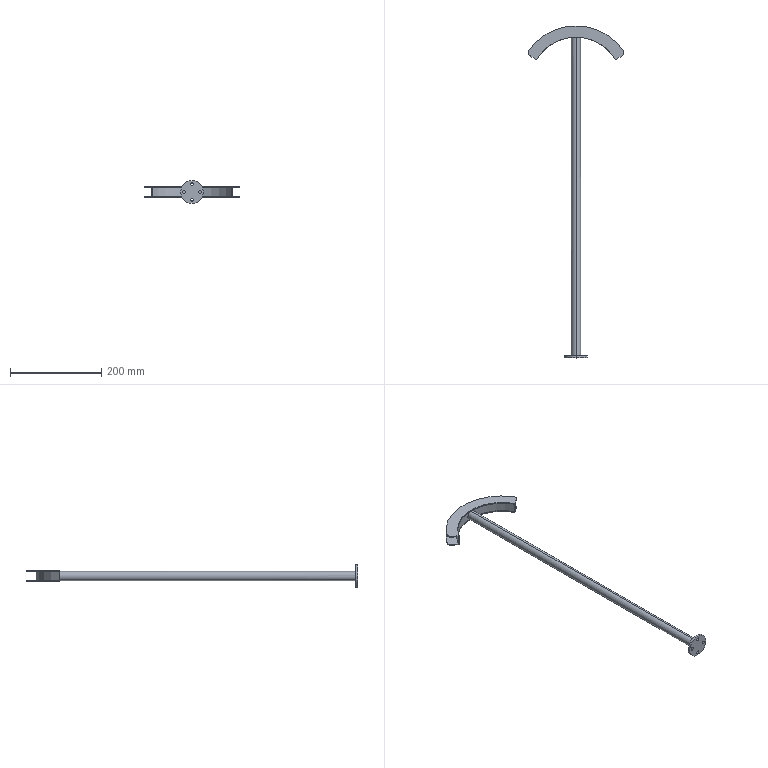Part | STEP file | TJ-DHQM-003-014 | 3 solids | 43 faces | box 208.431 x 730 x 50 mm | volume 102076 mm3 | cylinder 28 | plane 15 | commonest cylinder face diameters 6 x8 20 x8 200 x5 17 x2 50 x2 250 x2
STEP:
#1=CARTESIAN_POINT('',(104.216,65.942,-2.));
#2=VERTEX_POINT('',#1);
#3=CARTESIAN_POINT('',(99.216,57.282,-2.));
#4=VERTEX_POINT('',#3);
#5=CARTESIAN_POINT('',(94.216,65.942,-2.));
#6=DIRECTION('',(0.,0.,-1.));
#7=DIRECTION('',(-1.,0.,0.));
#8=AXIS2_PLACEMENT_3D('',#5,#6,#7);
#9=CIRCLE('',#8,10.);
#10=EDGE_CURVE('',#2,#4,#9,.T.);
#11=ORIENTED_EDGE('',*,*,#10,.F.);
#12=CARTESIAN_POINT('',(104.216,65.942,0.));
#13=VERTEX_POINT('',#12);
#14=CARTESIAN_POINT('',(104.216,65.942,-2.));
#15=DIRECTION('',(0.,0.,1.));
#16=VECTOR('',#15,1000.);
#17=LINE('',#14,#16);
#18=EDGE_CURVE('',#2,#13,#17,.T.);
#19=ORIENTED_EDGE('',*,*,#18,.T.);
#20=CARTESIAN_POINT('',(99.216,57.282,0.));
#21=VERTEX_POINT('',#20);
#22=CARTESIAN_POINT('',(94.216,65.942,0.));
#23=DIRECTION('',(0.,0.,1.));
#24=DIRECTION('',(-1.,0.,0.));
#25=AXIS2_PLACEMENT_3D('',#22,#23,#24);
#26=CIRCLE('',#25,10.);
#27=EDGE_CURVE('',#21,#13,#26,.T.);
#28=ORIENTED_EDGE('',*,*,#27,.F.);
#29=CARTESIAN_POINT('',(99.216,57.282,-2.));
#30=DIRECTION('',(0.,0.,1.));
#31=VECTOR('',#30,1000.);
#32=LINE('',#29,#31);
#33=EDGE_CURVE('',#4,#21,#32,.T.);
#34=ORIENTED_EDGE('',*,*,#33,.F.);
#35=EDGE_LOOP('',(#11,#19,#28,#34));
#36=FACE_OUTER_BOUND('',#35,.T.);
#37=CARTESIAN_POINT('',(94.216,65.942,-2.));
#38=DIRECTION('',(0.,0.,1.));
#39=DIRECTION('',(1.,0.,0.));
#40=AXIS2_PLACEMENT_3D('',#37,#38,#39);
#41=CYLINDRICAL_SURFACE('',#40,10.);
#42=ADVANCED_FACE('',(#36),#41,.T.);
#43=CARTESIAN_POINT('',(-102.408,71.677,0.));
#44=VERTEX_POINT('',#43);
#45=CARTESIAN_POINT('',(102.408,71.677,0.));
#46=VERTEX_POINT('',#45);
#47=CARTESIAN_POINT('',(0.,0.,0.));
#48=DIRECTION('',(0.,0.,-1.));
#49=DIRECTION('',(-1.,0.,0.));
#50=AXIS2_PLACEMENT_3D('',#47,#48,#49);
#51=CIRCLE('',#50,125.);
#52=EDGE_CURVE('',#44,#46,#51,.T.);
#53=ORIENTED_EDGE('',*,*,#52,.T.);
#54=CARTESIAN_POINT('',(102.408,71.677,-2.));
#55=VERTEX_POINT('',#54);
#56=CARTESIAN_POINT('',(102.408,71.677,-2.));
#57=DIRECTION('',(0.,0.,-1.));
#58=VECTOR('',#57,1000.);
#59=LINE('',#56,#58);
#60=EDGE_CURVE('',#46,#55,#59,.T.);
#61=ORIENTED_EDGE('',*,*,#60,.T.);
#62=CARTESIAN_POINT('',(-102.408,71.677,-2.));
#63=VERTEX_POINT('',#62);
#64=CARTESIAN_POINT('',(0.,0.,-2.));
#65=DIRECTION('',(0.,0.,-1.));
#66=DIRECTION('',(-1.,0.,0.));
#67=AXIS2_PLACEMENT_3D('',#64,#65,#66);
#68=CIRCLE('',#67,125.);
#69=EDGE_CURVE('',#63,#55,#68,.T.);
#70=ORIENTED_EDGE('',*,*,#69,.F.);
#71=CARTESIAN_POINT('',(-102.408,71.677,-2.));
#72=DIRECTION('',(0.,0.,1.));
#73=VECTOR('',#72,1000.);
#74=LINE('',#71,#73);
#75=EDGE_CURVE('',#63,#44,#74,.T.);
#76=ORIENTED_EDGE('',*,*,#75,.T.);
#77=EDGE_LOOP('',(#53,#61,#70,#76));
#78=FACE_OUTER_BOUND('',#77,.T.);
#79=CARTESIAN_POINT('',(0.,0.,-2.));
#80=DIRECTION('',(0.,0.,1.));
#81=DIRECTION('',(1.,0.,0.));
#82=AXIS2_PLACEMENT_3D('',#79,#80,#81);
#83=CYLINDRICAL_SURFACE('',#82,125.);
#84=ADVANCED_FACE('',(#78),#83,.T.);
#85=CARTESIAN_POINT('',(86.603,50.,-2.));
#86=VERTEX_POINT('',#85);
#87=CARTESIAN_POINT('',(108.253,62.5,-2.));
#88=DIRECTION('',(-0.866,-0.5,0.));
#89=VECTOR('',#88,1000.);
#90=LINE('',#87,#89);
#91=EDGE_CURVE('',#4,#86,#90,.T.);
#92=ORIENTED_EDGE('',*,*,#91,.F.);
#93=ORIENTED_EDGE('',*,*,#33,.T.);
#94=CARTESIAN_POINT('',(86.603,50.,0.));
#95=VERTEX_POINT('',#94);
#96=CARTESIAN_POINT('',(108.253,62.5,0.));
#97=DIRECTION('',(-0.866,-0.5,0.));
#98=VECTOR('',#97,1000.);
#99=LINE('',#96,#98);
#100=EDGE_CURVE('',#21,#95,#99,.T.);
#101=ORIENTED_EDGE('',*,*,#100,.T.);
#102=CARTESIAN_POINT('',(86.603,50.,-2.));
#103=DIRECTION('',(0.,0.,1.));
#104=VECTOR('',#103,1000.);
#105=LINE('',#102,#104);
#106=EDGE_CURVE('',#86,#95,#105,.T.);
#107=ORIENTED_EDGE('',*,*,#106,.F.);
#108=EDGE_LOOP('',(#92,#93,#101,#107));
#109=FACE_OUTER_BOUND('',#108,.T.);
#110=CARTESIAN_POINT('',(108.253,62.5,-2.));
#111=DIRECTION('',(-0.5,0.866,0.));
#112=DIRECTION('',(-0.866,-0.5,0.));
#113=AXIS2_PLACEMENT_3D('',#110,#111,#112);
#114=PLANE('',#113);
#115=ADVANCED_FACE('',(#109),#114,.F.);
#116=CARTESIAN_POINT('',(-86.603,50.,0.));
#117=VERTEX_POINT('',#116);
#118=CARTESIAN_POINT('',(0.,0.,0.));
#119=DIRECTION('',(0.,0.,1.));
#120=DIRECTION('',(-1.,0.,0.));
#121=AXIS2_PLACEMENT_3D('',#118,#119,#120);
#122=CIRCLE('',#121,100.);
#123=EDGE_CURVE('',#95,#117,#122,.T.);
#124=ORIENTED_EDGE('',*,*,#123,.T.);
#125=CARTESIAN_POINT('',(-86.603,50.,-2.));
#126=VERTEX_POINT('',#125);
#127=CARTESIAN_POINT('',(-86.603,50.,-2.));
#128=DIRECTION('',(0.,0.,1.));
#129=VECTOR('',#128,1000.);
#130=LINE('',#127,#129);
#131=EDGE_CURVE('',#126,#117,#130,.T.);
#132=ORIENTED_EDGE('',*,*,#131,.F.);
#133=CARTESIAN_POINT('',(0.,0.,-2.));
#134=DIRECTION('',(0.,0.,1.));
#135=DIRECTION('',(-1.,0.,0.));
#136=AXIS2_PLACEMENT_3D('',#133,#134,#135);
#137=CIRCLE('',#136,100.);
#138=EDGE_CURVE('',#86,#126,#137,.T.);
#139=ORIENTED_EDGE('',*,*,#138,.F.);
#140=ORIENTED_EDGE('',*,*,#106,.T.);
#141=EDGE_LOOP('',(#124,#132,#139,#140));
#142=FACE_OUTER_BOUND('',#141,.T.);
#143=CARTESIAN_POINT('',(0.,0.,-2.));
#144=DIRECTION('',(0.,0.,1.));
#145=DIRECTION('',(1.,0.,0.));
#146=AXIS2_PLACEMENT_3D('',#143,#144,#145);
#147=CYLINDRICAL_SURFACE('',#146,100.);
#148=ADVANCED_FACE('',(#142),#147,.F.);
#149=CARTESIAN_POINT('',(-99.216,57.282,0.));
#150=VERTEX_POINT('',#149);
#151=CARTESIAN_POINT('',(-86.603,50.,0.));
#152=DIRECTION('',(-0.866,0.5,0.));
#153=VECTOR('',#152,1000.);
#154=LINE('',#151,#153);
#155=EDGE_CURVE('',#117,#150,#154,.T.);
#156=ORIENTED_EDGE('',*,*,#155,.T.);
#157=CARTESIAN_POINT('',(-99.216,57.282,-2.));
#158=VERTEX_POINT('',#157);
#159=CARTESIAN_POINT('',(-99.216,57.282,-2.));
#160=DIRECTION('',(0.,0.,-1.));
#161=VECTOR('',#160,1000.);
#162=LINE('',#159,#161);
#163=EDGE_CURVE('',#150,#158,#162,.T.);
#164=ORIENTED_EDGE('',*,*,#163,.T.);
#165=CARTESIAN_POINT('',(-86.603,50.,-2.));
#166=DIRECTION('',(-0.866,0.5,0.));
#167=VECTOR('',#166,1000.);
#168=LINE('',#165,#167);
#169=EDGE_CURVE('',#126,#158,#168,.T.);
#170=ORIENTED_EDGE('',*,*,#169,.F.);
#171=ORIENTED_EDGE('',*,*,#131,.T.);
#172=EDGE_LOOP('',(#156,#164,#170,#171));
#173=FACE_OUTER_BOUND('',#172,.T.);
#174=CARTESIAN_POINT('',(-86.603,50.,-2.));
#175=DIRECTION('',(0.5,0.866,0.));
#176=DIRECTION('',(-0.866,0.5,0.));
#177=AXIS2_PLACEMENT_3D('',#174,#175,#176);
#178=PLANE('',#177);
#179=ADVANCED_FACE('',(#173),#178,.F.);
#180=ORIENTED_EDGE('',*,*,#69,.T.);
#181=CARTESIAN_POINT('',(94.216,65.942,-2.));
#182=DIRECTION('',(0.,0.,-1.));
#183=DIRECTION('',(-1.,0.,0.));
#184=AXIS2_PLACEMENT_3D('',#181,#182,#183);
#185=CIRCLE('',#184,10.);
#186=EDGE_CURVE('',#55,#2,#185,.T.);
#187=ORIENTED_EDGE('',*,*,#186,.T.);
#188=ORIENTED_EDGE('',*,*,#10,.T.);
#189=ORIENTED_EDGE('',*,*,#91,.T.);
#190=ORIENTED_EDGE('',*,*,#138,.T.);
#191=ORIENTED_EDGE('',*,*,#169,.T.);
#192=CARTESIAN_POINT('',(-94.216,65.942,-2.));
#193=DIRECTION('',(0.,0.,-1.));
#194=DIRECTION('',(-1.,0.,0.));
#195=AXIS2_PLACEMENT_3D('',#192,#193,#194);
#196=CIRCLE('',#195,10.);
#197=EDGE_CURVE('',#158,#63,#196,.T.);
#198=ORIENTED_EDGE('',*,*,#197,.T.);
#199=EDGE_LOOP('',(#180,#187,#188,#189,#190,#191,#198));
#200=FACE_OUTER_BOUND('',#199,.T.);
#201=CARTESIAN_POINT('',(0.,0.,-2.));
#202=DIRECTION('',(0.,0.,-1.));
#203=DIRECTION('',(-1.,0.,0.));
#204=AXIS2_PLACEMENT_3D('',#201,#202,#203);
#205=PLANE('',#204);
#206=ADVANCED_FACE('',(#200),#205,.T.);
#207=ORIENTED_EDGE('',*,*,#100,.F.);
#208=ORIENTED_EDGE('',*,*,#27,.T.);
#209=CARTESIAN_POINT('',(94.216,65.942,0.));
#210=DIRECTION('',(0.,0.,1.));
#211=DIRECTION('',(-1.,0.,0.));
#212=AXIS2_PLACEMENT_3D('',#209,#210,#211);
#213=CIRCLE('',#212,10.);
#214=EDGE_CURVE('',#13,#46,#213,.T.);
#215=ORIENTED_EDGE('',*,*,#214,.T.);
#216=ORIENTED_EDGE('',*,*,#52,.F.);
#217=CARTESIAN_POINT('',(-94.216,65.942,0.));
#218=DIRECTION('',(0.,0.,1.));
#219=DIRECTION('',(-1.,0.,0.));
#220=AXIS2_PLACEMENT_3D('',#217,#218,#219);
#221=CIRCLE('',#220,10.);
#222=EDGE_CURVE('',#44,#150,#221,.T.);
#223=ORIENTED_EDGE('',*,*,#222,.T.);
#224=ORIENTED_EDGE('',*,*,#155,.F.);
#225=ORIENTED_EDGE('',*,*,#123,.F.);
#226=EDGE_LOOP('',(#207,#208,#215,#216,#223,#224,#225));
#227=FACE_OUTER_BOUND('',#226,.T.);
#228=CARTESIAN_POINT('',(0.,0.,0.));
#229=DIRECTION('',(0.,0.,-1.));
#230=DIRECTION('',(-1.,0.,0.));
#231=AXIS2_PLACEMENT_3D('',#228,#229,#230);
#232=PLANE('',#231);
#233=ADVANCED_FACE('',(#227),#232,.F.);
#234=ORIENTED_EDGE('',*,*,#18,.F.);
#235=ORIENTED_EDGE('',*,*,#186,.F.);
#236=ORIENTED_EDGE('',*,*,#60,.F.);
#237=ORIENTED_EDGE('',*,*,#214,.F.);
#238=EDGE_LOOP('',(#234,#235,#236,#237));
#239=FACE_OUTER_BOUND('',#238,.T.);
#240=CARTESIAN_POINT('',(94.216,65.942,-2.));
#241=DIRECTION('',(0.,0.,1.));
#242=DIRECTION('',(1.,0.,0.));
#243=AXIS2_PLACEMENT_3D('',#240,#241,#242);
#244=CYLINDRICAL_SURFACE('',#243,10.);
#245=ADVANCED_FACE('',(#239),#244,.T.);
#246=ORIENTED_EDGE('',*,*,#197,.F.);
#247=ORIENTED_EDGE('',*,*,#163,.F.);
#248=ORIENTED_EDGE('',*,*,#222,.F.);
#249=ORIENTED_EDGE('',*,*,#75,.F.);
#250=EDGE_LOOP('',(#246,#247,#248,#249));
#251=FACE_OUTER_BOUND('',#250,.T.);
#252=CARTESIAN_POINT('',(-94.216,65.942,-2.));
#253=DIRECTION('',(0.,0.,1.));
#254=DIRECTION('',(1.,0.,0.));
#255=AXIS2_PLACEMENT_3D('',#252,#253,#254);
#256=CYLINDRICAL_SURFACE('',#255,10.);
#257=ADVANCED_FACE('',(#251),#256,.T.);
#258=CLOSED_SHELL('',(#42,#84,#115,#148,#179,#206,#233,#245,#257));
#259=MANIFOLD_SOLID_BREP('',#258);
#260=CARTESIAN_POINT('',(-104.216,65.942,22.));
#261=VERTEX_POINT('',#260);
#262=CARTESIAN_POINT('',(-99.216,57.282,22.));
#263=VERTEX_POINT('',#262);
#264=CARTESIAN_POINT('',(-94.216,65.942,22.));
#265=DIRECTION('',(0.,0.,1.));
#266=DIRECTION('',(1.,0.,0.));
#267=AXIS2_PLACEMENT_3D('',#264,#265,#266);
#268=CIRCLE('',#267,10.);
#269=EDGE_CURVE('',#261,#263,#268,.T.);
#270=ORIENTED_EDGE('',*,*,#269,.F.);
#271=CARTESIAN_POINT('',(-104.216,65.942,20.));
#272=VERTEX_POINT('',#271);
#273=CARTESIAN_POINT('',(-104.216,65.942,22.));
#274=DIRECTION('',(0.,0.,-1.));
#275=VECTOR('',#274,1000.);
#276=LINE('',#273,#275);
#277=EDGE_CURVE('',#261,#272,#276,.T.);
#278=ORIENTED_EDGE('',*,*,#277,.T.);
#279=CARTESIAN_POINT('',(-99.216,57.282,20.));
#280=VERTEX_POINT('',#279);
#281=CARTESIAN_POINT('',(-94.216,65.942,20.));
#282=DIRECTION('',(0.,0.,-1.));
#283=DIRECTION('',(1.,0.,0.));
#284=AXIS2_PLACEMENT_3D('',#281,#282,#283);
#285=CIRCLE('',#284,10.);
#286=EDGE_CURVE('',#280,#272,#285,.T.);
#287=ORIENTED_EDGE('',*,*,#286,.F.);
#288=CARTESIAN_POINT('',(-99.216,57.282,22.));
#289=DIRECTION('',(0.,0.,-1.));
#290=VECTOR('',#289,1000.);
#291=LINE('',#288,#290);
#292=EDGE_CURVE('',#263,#280,#291,.T.);
#293=ORIENTED_EDGE('',*,*,#292,.F.);
#294=EDGE_LOOP('',(#270,#278,#287,#293));
#295=FACE_OUTER_BOUND('',#294,.T.);
#296=CARTESIAN_POINT('',(-94.216,65.942,22.));
#297=DIRECTION('',(0.,0.,-1.));
#298=DIRECTION('',(-1.,0.,0.));
#299=AXIS2_PLACEMENT_3D('',#296,#297,#298);
#300=CYLINDRICAL_SURFACE('',#299,10.);
#301=ADVANCED_FACE('',(#295),#300,.T.);
#302=CARTESIAN_POINT('',(102.408,71.677,20.));
#303=VERTEX_POINT('',#302);
#304=CARTESIAN_POINT('',(-102.408,71.677,20.));
#305=VERTEX_POINT('',#304);
#306=CARTESIAN_POINT('',(0.,0.,20.));
#307=DIRECTION('',(0.,0.,1.));
#308=DIRECTION('',(1.,0.,0.));
#309=AXIS2_PLACEMENT_3D('',#306,#307,#308);
#310=CIRCLE('',#309,125.);
#311=EDGE_CURVE('',#303,#305,#310,.T.);
#312=ORIENTED_EDGE('',*,*,#311,.T.);
#313=CARTESIAN_POINT('',(-102.408,71.677,22.));
#314=VERTEX_POINT('',#313);
#315=CARTESIAN_POINT('',(-102.408,71.677,22.));
#316=DIRECTION('',(0.,0.,1.));
#317=VECTOR('',#316,1000.);
#318=LINE('',#315,#317);
#319=EDGE_CURVE('',#305,#314,#318,.T.);
#320=ORIENTED_EDGE('',*,*,#319,.T.);
#321=CARTESIAN_POINT('',(102.408,71.677,22.));
#322=VERTEX_POINT('',#321);
#323=CARTESIAN_POINT('',(0.,0.,22.));
#324=DIRECTION('',(0.,0.,1.));
#325=DIRECTION('',(1.,0.,0.));
#326=AXIS2_PLACEMENT_3D('',#323,#324,#325);
#327=CIRCLE('',#326,125.);
#328=EDGE_CURVE('',#322,#314,#327,.T.);
#329=ORIENTED_EDGE('',*,*,#328,.F.);
#330=CARTESIAN_POINT('',(102.408,71.677,22.));
#331=DIRECTION('',(0.,0.,-1.));
#332=VECTOR('',#331,1000.);
#333=LINE('',#330,#332);
#334=EDGE_CURVE('',#322,#303,#333,.T.);
#335=ORIENTED_EDGE('',*,*,#334,.T.);
#336=EDGE_LOOP('',(#312,#320,#329,#335));
#337=FACE_OUTER_BOUND('',#336,.T.);
#338=CARTESIAN_POINT('',(0.,0.,22.));
#339=DIRECTION('',(0.,0.,-1.));
#340=DIRECTION('',(-1.,0.,0.));
#341=AXIS2_PLACEMENT_3D('',#338,#339,#340);
#342=CYLINDRICAL_SURFACE('',#341,125.);
#343=ADVANCED_FACE('',(#337),#342,.T.);
#344=CARTESIAN_POINT('',(-86.603,50.,22.));
#345=VERTEX_POINT('',#344);
#346=CARTESIAN_POINT('',(-108.253,62.5,22.));
#347=DIRECTION('',(0.866,-0.5,0.));
#348=VECTOR('',#347,1000.);
#349=LINE('',#346,#348);
#350=EDGE_CURVE('',#263,#345,#349,.T.);
#351=ORIENTED_EDGE('',*,*,#350,.F.);
#352=ORIENTED_EDGE('',*,*,#292,.T.);
#353=CARTESIAN_POINT('',(-86.603,50.,20.));
#354=VERTEX_POINT('',#353);
#355=CARTESIAN_POINT('',(-108.253,62.5,20.));
#356=DIRECTION('',(0.866,-0.5,0.));
#357=VECTOR('',#356,1000.);
#358=LINE('',#355,#357);
#359=EDGE_CURVE('',#280,#354,#358,.T.);
#360=ORIENTED_EDGE('',*,*,#359,.T.);
#361=CARTESIAN_POINT('',(-86.603,50.,22.));
#362=DIRECTION('',(0.,0.,-1.));
#363=VECTOR('',#362,1000.);
#364=LINE('',#361,#363);
#365=EDGE_CURVE('',#345,#354,#364,.T.);
#366=ORIENTED_EDGE('',*,*,#365,.F.);
#367=EDGE_LOOP('',(#351,#352,#360,#366));
#368=FACE_OUTER_BOUND('',#367,.T.);
#369=CARTESIAN_POINT('',(-108.253,62.5,22.));
#370=DIRECTION('',(0.5,0.866,0.));
#371=DIRECTION('',(-0.866,0.5,0.));
#372=AXIS2_PLACEMENT_3D('',#369,#370,#371);
#373=PLANE('',#372);
#374=ADVANCED_FACE('',(#368),#373,.F.);
#375=CARTESIAN_POINT('',(86.603,50.,20.));
#376=VERTEX_POINT('',#375);
#377=CARTESIAN_POINT('',(0.,0.,20.));
#378=DIRECTION('',(0.,0.,-1.));
#379=DIRECTION('',(1.,0.,0.));
#380=AXIS2_PLACEMENT_3D('',#377,#378,#379);
#381=CIRCLE('',#380,100.);
#382=EDGE_CURVE('',#354,#376,#381,.T.);
#383=ORIENTED_EDGE('',*,*,#382,.T.);
#384=CARTESIAN_POINT('',(86.603,50.,22.));
#385=VERTEX_POINT('',#384);
#386=CARTESIAN_POINT('',(86.603,50.,22.));
#387=DIRECTION('',(0.,0.,-1.));
#388=VECTOR('',#387,1000.);
#389=LINE('',#386,#388);
#390=EDGE_CURVE('',#385,#376,#389,.T.);
#391=ORIENTED_EDGE('',*,*,#390,.F.);
#392=CARTESIAN_POINT('',(0.,0.,22.));
#393=DIRECTION('',(0.,0.,-1.));
#394=DIRECTION('',(1.,0.,0.));
#395=AXIS2_PLACEMENT_3D('',#392,#393,#394);
#396=CIRCLE('',#395,100.);
#397=EDGE_CURVE('',#345,#385,#396,.T.);
#398=ORIENTED_EDGE('',*,*,#397,.F.);
#399=ORIENTED_EDGE('',*,*,#365,.T.);
#400=EDGE_LOOP('',(#383,#391,#398,#399));
#401=FACE_OUTER_BOUND('',#400,.T.);
#402=CARTESIAN_POINT('',(0.,0.,22.));
#403=DIRECTION('',(0.,0.,-1.));
#404=DIRECTION('',(-1.,0.,0.));
#405=AXIS2_PLACEMENT_3D('',#402,#403,#404);
#406=CYLINDRICAL_SURFACE('',#405,100.);
#407=ADVANCED_FACE('',(#401),#406,.F.);
#408=CARTESIAN_POINT('',(99.216,57.282,20.));
#409=VERTEX_POINT('',#408);
#410=CARTESIAN_POINT('',(86.603,50.,20.));
#411=DIRECTION('',(0.866,0.5,0.));
#412=VECTOR('',#411,1000.);
#413=LINE('',#410,#412);
#414=EDGE_CURVE('',#376,#409,#413,.T.);
#415=ORIENTED_EDGE('',*,*,#414,.T.);
#416=CARTESIAN_POINT('',(99.216,57.282,22.));
#417=VERTEX_POINT('',#416);
#418=CARTESIAN_POINT('',(99.216,57.282,22.));
#419=DIRECTION('',(0.,0.,1.));
#420=VECTOR('',#419,1000.);
#421=LINE('',#418,#420);
#422=EDGE_CURVE('',#409,#417,#421,.T.);
#423=ORIENTED_EDGE('',*,*,#422,.T.);
#424=CARTESIAN_POINT('',(86.603,50.,22.));
#425=DIRECTION('',(0.866,0.5,0.));
#426=VECTOR('',#425,1000.);
#427=LINE('',#424,#426);
#428=EDGE_CURVE('',#385,#417,#427,.T.);
#429=ORIENTED_EDGE('',*,*,#428,.F.);
#430=ORIENTED_EDGE('',*,*,#390,.T.);
#431=EDGE_LOOP('',(#415,#423,#429,#430));
#432=FACE_OUTER_BOUND('',#431,.T.);
#433=CARTESIAN_POINT('',(86.603,50.,22.));
#434=DIRECTION('',(-0.5,0.866,0.));
#435=DIRECTION('',(-0.866,-0.5,0.));
#436=AXIS2_PLACEMENT_3D('',#433,#434,#435);
#437=PLANE('',#436);
#438=ADVANCED_FACE('',(#432),#437,.F.);
#439=ORIENTED_EDGE('',*,*,#328,.T.);
#440=CARTESIAN_POINT('',(-94.216,65.942,22.));
#441=DIRECTION('',(0.,0.,1.));
#442=DIRECTION('',(1.,0.,0.));
#443=AXIS2_PLACEMENT_3D('',#440,#441,#442);
#444=CIRCLE('',#443,10.);
#445=EDGE_CURVE('',#314,#261,#444,.T.);
#446=ORIENTED_EDGE('',*,*,#445,.T.);
#447=ORIENTED_EDGE('',*,*,#269,.T.);
#448=ORIENTED_EDGE('',*,*,#350,.T.);
#449=ORIENTED_EDGE('',*,*,#397,.T.);
#450=ORIENTED_EDGE('',*,*,#428,.T.);
#451=CARTESIAN_POINT('',(94.216,65.942,22.));
#452=DIRECTION('',(0.,0.,1.));
#453=DIRECTION('',(1.,0.,0.));
#454=AXIS2_PLACEMENT_3D('',#451,#452,#453);
#455=CIRCLE('',#454,10.);
#456=EDGE_CURVE('',#417,#322,#455,.T.);
#457=ORIENTED_EDGE('',*,*,#456,.T.);
#458=EDGE_LOOP('',(#439,#446,#447,#448,#449,#450,#457));
#459=FACE_OUTER_BOUND('',#458,.T.);
#460=CARTESIAN_POINT('',(0.,0.,22.));
#461=DIRECTION('',(0.,0.,1.));
#462=DIRECTION('',(1.,0.,0.));
#463=AXIS2_PLACEMENT_3D('',#460,#461,#462);
#464=PLANE('',#463);
#465=ADVANCED_FACE('',(#459),#464,.T.);
#466=ORIENTED_EDGE('',*,*,#359,.F.);
#467=ORIENTED_EDGE('',*,*,#286,.T.);
#468=CARTESIAN_POINT('',(-94.216,65.942,20.));
#469=DIRECTION('',(0.,0.,-1.));
#470=DIRECTION('',(1.,0.,0.));
#471=AXIS2_PLACEMENT_3D('',#468,#469,#470);
#472=CIRCLE('',#471,10.);
#473=EDGE_CURVE('',#272,#305,#472,.T.);
#474=ORIENTED_EDGE('',*,*,#473,.T.);
#475=ORIENTED_EDGE('',*,*,#311,.F.);
#476=CARTESIAN_POINT('',(94.216,65.942,20.));
#477=DIRECTION('',(0.,0.,-1.));
#478=DIRECTION('',(1.,0.,0.));
#479=AXIS2_PLACEMENT_3D('',#476,#477,#478);
#480=CIRCLE('',#479,10.);
#481=EDGE_CURVE('',#303,#409,#480,.T.);
#482=ORIENTED_EDGE('',*,*,#481,.T.);
#483=ORIENTED_EDGE('',*,*,#414,.F.);
#484=ORIENTED_EDGE('',*,*,#382,.F.);
#485=EDGE_LOOP('',(#466,#467,#474,#475,#482,#483,#484));
#486=FACE_OUTER_BOUND('',#485,.T.);
#487=CARTESIAN_POINT('',(0.,0.,20.));
#488=DIRECTION('',(0.,0.,1.));
#489=DIRECTION('',(1.,0.,0.));
#490=AXIS2_PLACEMENT_3D('',#487,#488,#489);
#491=PLANE('',#490);
#492=ADVANCED_FACE('',(#486),#491,.F.);
#493=ORIENTED_EDGE('',*,*,#277,.F.);
#494=ORIENTED_EDGE('',*,*,#445,.F.);
#495=ORIENTED_EDGE('',*,*,#319,.F.);
#496=ORIENTED_EDGE('',*,*,#473,.F.);
#497=EDGE_LOOP('',(#493,#494,#495,#496));
#498=FACE_OUTER_BOUND('',#497,.T.);
#499=CARTESIAN_POINT('',(-94.216,65.942,22.));
#500=DIRECTION('',(0.,0.,-1.));
#501=DIRECTION('',(-1.,0.,0.));
#502=AXIS2_PLACEMENT_3D('',#499,#500,#501);
#503=CYLINDRICAL_SURFACE('',#502,10.);
#504=ADVANCED_FACE('',(#498),#503,.T.);
#505=ORIENTED_EDGE('',*,*,#456,.F.);
#506=ORIENTED_EDGE('',*,*,#422,.F.);
#507=ORIENTED_EDGE('',*,*,#481,.F.);
#508=ORIENTED_EDGE('',*,*,#334,.F.);
#509=EDGE_LOOP('',(#505,#506,#507,#508));
#510=FACE_OUTER_BOUND('',#509,.T.);
#511=CARTESIAN_POINT('',(94.216,65.942,22.));
#512=DIRECTION('',(0.,0.,-1.));
#513=DIRECTION('',(-1.,0.,0.));
#514=AXIS2_PLACEMENT_3D('',#511,#512,#513);
#515=CYLINDRICAL_SURFACE('',#514,10.);
#516=ADVANCED_FACE('',(#510),#515,.T.);
#517=CLOSED_SHELL('',(#301,#343,#374,#407,#438,#465,#492,#504,#516));
#518=MANIFOLD_SOLID_BREP('',#517);
#519=CARTESIAN_POINT('',(0.,-600.,30.5));
#520=VERTEX_POINT('',#519);
#521=CARTESIAN_POINT('',(0.,-600.,24.5));
#522=VERTEX_POINT('',#521);
#523=CARTESIAN_POINT('',(0.,-600.,27.5));
#524=DIRECTION('',(0.,-1.,0.));
#525=DIRECTION('',(0.,0.,-1.));
#526=AXIS2_PLACEMENT_3D('',#523,#524,#525);
#527=CIRCLE('',#526,3.);
#528=EDGE_CURVE('',#520,#522,#527,.T.);
#529=ORIENTED_EDGE('',*,*,#528,.F.);
#530=CARTESIAN_POINT('',(0.,-605.,30.5));
#531=VERTEX_POINT('',#530);
#532=CARTESIAN_POINT('',(0.,-595.,30.5));
#533=DIRECTION('',(0.,-1.,0.));
#534=VECTOR('',#533,1000.);
#535=LINE('',#532,#534);
#536=EDGE_CURVE('',#520,#531,#535,.T.);
#537=ORIENTED_EDGE('',*,*,#536,.T.);
#538=CARTESIAN_POINT('',(0.,-605.,24.5));
#539=VERTEX_POINT('',#538);
#540=CARTESIAN_POINT('',(0.,-605.,27.5));
#541=DIRECTION('',(0.,-1.,0.));
#542=DIRECTION('',(0.,0.,-1.));
#543=AXIS2_PLACEMENT_3D('',#540,#541,#542);
#544=CIRCLE('',#543,3.);
#545=EDGE_CURVE('',#531,#539,#544,.T.);
#546=ORIENTED_EDGE('',*,*,#545,.T.);
#547=CARTESIAN_POINT('',(0.,-595.,24.5));
#548=DIRECTION('',(0.,-1.,0.));
#549=VECTOR('',#548,1000.);
#550=LINE('',#547,#549);
#551=EDGE_CURVE('',#522,#539,#550,.T.);
#552=ORIENTED_EDGE('',*,*,#551,.F.);
#553=EDGE_LOOP('',(#529,#537,#546,#552));
#554=FACE_OUTER_BOUND('',#553,.T.);
#555=CARTESIAN_POINT('',(0.,-595.,27.5));
#556=DIRECTION('',(0.,-1.,0.));
#557=DIRECTION('',(0.,0.,-1.));
#558=AXIS2_PLACEMENT_3D('',#555,#556,#557);
#559=CYLINDRICAL_SURFACE('',#558,3.);
#560=ADVANCED_FACE('',(#554),#559,.F.);
#561=CARTESIAN_POINT('',(-17.5,-600.,13.));
#562=VERTEX_POINT('',#561);
#563=CARTESIAN_POINT('',(-17.5,-600.,7.));
#564=VERTEX_POINT('',#563);
#565=CARTESIAN_POINT('',(-17.5,-600.,10.));
#566=DIRECTION('',(0.,-1.,0.));
#567=DIRECTION('',(0.,0.,-1.));
#568=AXIS2_PLACEMENT_3D('',#565,#566,#567);
#569=CIRCLE('',#568,3.);
#570=EDGE_CURVE('',#562,#564,#569,.T.);
#571=ORIENTED_EDGE('',*,*,#570,.F.);
#572=CARTESIAN_POINT('',(-17.5,-605.,13.));
#573=VERTEX_POINT('',#572);
#574=CARTESIAN_POINT('',(-17.5,-595.,13.));
#575=DIRECTION('',(0.,-1.,0.));
#576=VECTOR('',#575,1000.);
#577=LINE('',#574,#576);
#578=EDGE_CURVE('',#562,#573,#577,.T.);
#579=ORIENTED_EDGE('',*,*,#578,.T.);
#580=CARTESIAN_POINT('',(-17.5,-605.,7.));
#581=VERTEX_POINT('',#580);
#582=CARTESIAN_POINT('',(-17.5,-605.,10.));
#583=DIRECTION('',(0.,-1.,0.));
#584=DIRECTION('',(0.,0.,-1.));
#585=AXIS2_PLACEMENT_3D('',#582,#583,#584);
#586=CIRCLE('',#585,3.);
#587=EDGE_CURVE('',#573,#581,#586,.T.);
#588=ORIENTED_EDGE('',*,*,#587,.T.);
#589=CARTESIAN_POINT('',(-17.5,-595.,7.));
#590=DIRECTION('',(0.,-1.,0.));
#591=VECTOR('',#590,1000.);
#592=LINE('',#589,#591);
#593=EDGE_CURVE('',#564,#581,#592,.T.);
#594=ORIENTED_EDGE('',*,*,#593,.F.);
#595=EDGE_LOOP('',(#571,#579,#588,#594));
#596=FACE_OUTER_BOUND('',#595,.T.);
#597=CARTESIAN_POINT('',(-17.5,-595.,10.));
#598=DIRECTION('',(0.,-1.,0.));
#599=DIRECTION('',(0.,0.,-1.));
#600=AXIS2_PLACEMENT_3D('',#597,#598,#599);
#601=CYLINDRICAL_SURFACE('',#600,3.);
#602=ADVANCED_FACE('',(#596),#601,.F.);
#603=CARTESIAN_POINT('',(0.,-600.,-4.5));
#604=VERTEX_POINT('',#603);
#605=CARTESIAN_POINT('',(0.,-600.,-10.5));
#606=VERTEX_POINT('',#605);
#607=CARTESIAN_POINT('',(0.,-600.,-7.5));
#608=DIRECTION('',(0.,-1.,0.));
#609=DIRECTION('',(0.,0.,-1.));
#610=AXIS2_PLACEMENT_3D('',#607,#608,#609);
#611=CIRCLE('',#610,3.);
#612=EDGE_CURVE('',#604,#606,#611,.T.);
#613=ORIENTED_EDGE('',*,*,#612,.F.);
#614=CARTESIAN_POINT('',(0.,-605.,-4.5));
#615=VERTEX_POINT('',#614);
#616=CARTESIAN_POINT('',(0.,-595.,-4.5));
#617=DIRECTION('',(0.,-1.,0.));
#618=VECTOR('',#617,1000.);
#619=LINE('',#616,#618);
#620=EDGE_CURVE('',#604,#615,#619,.T.);
#621=ORIENTED_EDGE('',*,*,#620,.T.);
#622=CARTESIAN_POINT('',(0.,-605.,-10.5));
#623=VERTEX_POINT('',#622);
#624=CARTESIAN_POINT('',(0.,-605.,-7.5));
#625=DIRECTION('',(0.,-1.,0.));
#626=DIRECTION('',(0.,0.,-1.));
#627=AXIS2_PLACEMENT_3D('',#624,#625,#626);
#628=CIRCLE('',#627,3.);
#629=EDGE_CURVE('',#615,#623,#628,.T.);
#630=ORIENTED_EDGE('',*,*,#629,.T.);
#631=CARTESIAN_POINT('',(0.,-595.,-10.5));
#632=DIRECTION('',(0.,-1.,0.));
#633=VECTOR('',#632,1000.);
#634=LINE('',#631,#633);
#635=EDGE_CURVE('',#606,#623,#634,.T.);
#636=ORIENTED_EDGE('',*,*,#635,.F.);
#637=EDGE_LOOP('',(#613,#621,#630,#636));
#638=FACE_OUTER_BOUND('',#637,.T.);
#639=CARTESIAN_POINT('',(0.,-595.,-7.5));
#640=DIRECTION('',(0.,-1.,0.));
#641=DIRECTION('',(0.,0.,-1.));
#642=AXIS2_PLACEMENT_3D('',#639,#640,#641);
#643=CYLINDRICAL_SURFACE('',#642,3.);
#644=ADVANCED_FACE('',(#638),#643,.F.);
#645=CARTESIAN_POINT('',(17.5,-600.,13.));
#646=VERTEX_POINT('',#645);
#647=CARTESIAN_POINT('',(17.5,-600.,7.));
#648=VERTEX_POINT('',#647);
#649=CARTESIAN_POINT('',(17.5,-600.,10.));
#650=DIRECTION('',(0.,-1.,0.));
#651=DIRECTION('',(0.,0.,-1.));
#652=AXIS2_PLACEMENT_3D('',#649,#650,#651);
#653=CIRCLE('',#652,3.);
#654=EDGE_CURVE('',#646,#648,#653,.T.);
#655=ORIENTED_EDGE('',*,*,#654,.F.);
#656=CARTESIAN_POINT('',(17.5,-605.,13.));
#657=VERTEX_POINT('',#656);
#658=CARTESIAN_POINT('',(17.5,-595.,13.));
#659=DIRECTION('',(0.,-1.,0.));
#660=VECTOR('',#659,1000.);
#661=LINE('',#658,#660);
#662=EDGE_CURVE('',#646,#657,#661,.T.);
#663=ORIENTED_EDGE('',*,*,#662,.T.);
#664=CARTESIAN_POINT('',(17.5,-605.,7.));
#665=VERTEX_POINT('',#664);
#666=CARTESIAN_POINT('',(17.5,-605.,10.));
#667=DIRECTION('',(0.,-1.,0.));
#668=DIRECTION('',(0.,0.,-1.));
#669=AXIS2_PLACEMENT_3D('',#666,#667,#668);
#670=CIRCLE('',#669,3.);
#671=EDGE_CURVE('',#657,#665,#670,.T.);
#672=ORIENTED_EDGE('',*,*,#671,.T.);
#673=CARTESIAN_POINT('',(17.5,-595.,7.));
#674=DIRECTION('',(0.,-1.,0.));
#675=VECTOR('',#674,1000.);
#676=LINE('',#673,#675);
#677=EDGE_CURVE('',#648,#665,#676,.T.);
#678=ORIENTED_EDGE('',*,*,#677,.F.);
#679=EDGE_LOOP('',(#655,#663,#672,#678));
#680=FACE_OUTER_BOUND('',#679,.T.);
#681=CARTESIAN_POINT('',(17.5,-595.,10.));
#682=DIRECTION('',(0.,-1.,0.));
#683=DIRECTION('',(0.,0.,-1.));
#684=AXIS2_PLACEMENT_3D('',#681,#682,#683);
#685=CYLINDRICAL_SURFACE('',#684,3.);
#686=ADVANCED_FACE('',(#680),#685,.F.);
#687=CARTESIAN_POINT('',(0.,-605.,-15.));
#688=VERTEX_POINT('',#687);
#689=CARTESIAN_POINT('',(0.,-605.,35.));
#690=VERTEX_POINT('',#689);
#691=CARTESIAN_POINT('',(0.,-605.,10.));
#692=DIRECTION('',(0.,-1.,0.));
#693=DIRECTION('',(0.,0.,-1.));
#694=AXIS2_PLACEMENT_3D('',#691,#692,#693);
#695=CIRCLE('',#694,25.);
#696=EDGE_CURVE('',#688,#690,#695,.T.);
#697=ORIENTED_EDGE('',*,*,#696,.F.);
#698=CARTESIAN_POINT('',(0.,-600.,-15.));
#699=VERTEX_POINT('',#698);
#700=CARTESIAN_POINT('',(0.,-605.,-15.));
#701=DIRECTION('',(0.,1.,0.));
#702=VECTOR('',#701,1000.);
#703=LINE('',#700,#702);
#704=EDGE_CURVE('',#688,#699,#703,.T.);
#705=ORIENTED_EDGE('',*,*,#704,.T.);
#706=CARTESIAN_POINT('',(0.,-600.,35.));
#707=VERTEX_POINT('',#706);
#708=CARTESIAN_POINT('',(0.,-600.,10.));
#709=DIRECTION('',(0.,-1.,0.));
#710=DIRECTION('',(0.,0.,-1.));
#711=AXIS2_PLACEMENT_3D('',#708,#709,#710);
#712=CIRCLE('',#711,25.);
#713=EDGE_CURVE('',#699,#707,#712,.T.);
#714=ORIENTED_EDGE('',*,*,#713,.T.);
#715=CARTESIAN_POINT('',(0.,-605.,35.));
#716=DIRECTION('',(0.,1.,0.));
#717=VECTOR('',#716,1000.);
#718=LINE('',#715,#717);
#719=EDGE_CURVE('',#690,#707,#718,.T.);
#720=ORIENTED_EDGE('',*,*,#719,.F.);
#721=EDGE_LOOP('',(#697,#705,#714,#720));
#722=FACE_OUTER_BOUND('',#721,.T.);
#723=CARTESIAN_POINT('',(0.,-605.,10.));
#724=DIRECTION('',(0.,1.,0.));
#725=DIRECTION('',(0.,0.,1.));
#726=AXIS2_PLACEMENT_3D('',#723,#724,#725);
#727=CYLINDRICAL_SURFACE('',#726,25.);
#728=ADVANCED_FACE('',(#722),#727,.T.);
#729=CARTESIAN_POINT('',(0.,100.,0.));
#730=VERTEX_POINT('',#729);
#731=CARTESIAN_POINT('',(0.,100.,20.));
#732=VERTEX_POINT('',#731);
#733=CARTESIAN_POINT('',(0.,100.,0.));
#734=CARTESIAN_POINT('',(0.6612,100.,0.));
#735=CARTESIAN_POINT('',(1.311,99.993,0.06493));
#736=CARTESIAN_POINT('',(2.27,99.975,0.2557));
#737=CARTESIAN_POINT('',(2.587,99.967,0.3349));
#738=CARTESIAN_POINT('',(3.216,99.949,0.5255));
#739=CARTESIAN_POINT('',(3.528,99.938,0.6373));
#740=CARTESIAN_POINT('',(4.436,99.903,1.014));
#741=CARTESIAN_POINT('',(5.01,99.876,1.321));
#742=CARTESIAN_POINT('',(5.826,99.831,1.866));
#743=CARTESIAN_POINT('',(6.091,99.815,2.062));
#744=CARTESIAN_POINT('',(6.6,99.782,2.48));
#745=CARTESIAN_POINT('',(6.842,99.766,2.7));
#746=CARTESIAN_POINT('',(7.533,99.717,3.391));
#747=CARTESIAN_POINT('',(7.947,99.684,3.895));
#748=CARTESIAN_POINT('',(8.495,99.639,4.715));
#749=CARTESIAN_POINT('',(8.666,99.624,4.998));
#750=CARTESIAN_POINT('',(8.974,99.597,5.575));
#751=CARTESIAN_POINT('',(9.253,99.571,6.165));
#752=CARTESIAN_POINT('',(9.473,99.55,6.779));
#753=CARTESIAN_POINT('',(9.663,99.532,7.405));
#754=CARTESIAN_POINT('',(9.744,99.524,7.726));
#755=CARTESIAN_POINT('',(9.936,99.505,8.695));
#756=CARTESIAN_POINT('',(10.,99.499,9.344));
#757=CARTESIAN_POINT('',(10.,99.499,10.323));
#758=CARTESIAN_POINT('',(9.984,99.5,10.65));
#759=CARTESIAN_POINT('',(9.92,99.507,11.306));
#760=CARTESIAN_POINT('',(9.871,99.512,11.633));
#761=CARTESIAN_POINT('',(9.68,99.531,12.595));
#762=CARTESIAN_POINT('',(9.491,99.549,13.219));
#763=CARTESIAN_POINT('',(9.115,99.584,14.127));
#764=CARTESIAN_POINT('',(8.973,99.597,14.427));
#765=CARTESIAN_POINT('',(8.663,99.624,15.006));
#766=CARTESIAN_POINT('',(8.495,99.639,15.286));
#767=CARTESIAN_POINT('',(7.952,99.684,16.098));
#768=CARTESIAN_POINT('',(7.539,99.717,16.603));
#769=CARTESIAN_POINT('',(6.605,99.783,17.537));
#770=CARTESIAN_POINT('',(6.1,99.815,17.95));
#771=CARTESIAN_POINT('',(5.288,99.86,18.493));
#772=CARTESIAN_POINT('',(5.009,99.875,18.662));
#773=CARTESIAN_POINT('',(4.43,99.902,18.971));
#774=CARTESIAN_POINT('',(4.13,99.915,19.113));
#775=CARTESIAN_POINT('',(3.222,99.95,19.489));
#776=CARTESIAN_POINT('',(2.598,99.968,19.679));
#777=CARTESIAN_POINT('',(1.637,99.987,19.871));
#778=CARTESIAN_POINT('',(1.31,99.992,19.919));
#779=CARTESIAN_POINT('',(0.6538,99.998,19.984));
#780=CARTESIAN_POINT('',(0.3264,100.,20.));
#781=CARTESIAN_POINT('',(0.,100.,20.));
#782=B_SPLINE_CURVE_WITH_KNOTS('',3,(#733,#734,#735,#736,#737,#738,#739,#740,#741,#742,#743,#744,#745,#746,#747,#748,#749,#750,#751,#752,#753,#754,#755,#756,#757,#758,#759,#760,#761,#762,#763,#764,#765,#766,#767,#768,#769,#770,#771,#772,#773,#774,#775,#776,#777,#778,#779,#780,#781),.UNSPECIFIED.,.F.,.F.,(4,2,2,2,2,2,2,2,2,1,2,2,2,2,2,2,2,2,2,2,2,2,2,2,4),(0.,0.001955,0.002933,0.003911,0.005866,0.006843,0.007821,0.009776,0.01075,0.01173,0.01271,0.01369,0.01564,0.01662,0.0176,0.01955,0.02053,0.02151,0.02346,0.02542,0.0264,0.02737,0.02933,0.03031,0.03128),.UNSPECIFIED.);
#783=EDGE_CURVE('',#730,#732,#782,.T.);
#784=ORIENTED_EDGE('',*,*,#783,.T.);
#785=CARTESIAN_POINT('',(0.,-600.,20.));
#786=VERTEX_POINT('',#785);
#787=CARTESIAN_POINT('',(0.,125.001,20.));
#788=DIRECTION('',(0.,-1.,0.));
#789=VECTOR('',#788,1000.);
#790=LINE('',#787,#789);
#791=EDGE_CURVE('',#732,#786,#790,.T.);
#792=ORIENTED_EDGE('',*,*,#791,.T.);
#793=CARTESIAN_POINT('',(0.,-600.,0.));
#794=VERTEX_POINT('',#793);
#795=CARTESIAN_POINT('',(0.,-600.,10.));
#796=DIRECTION('',(0.,1.,0.));
#797=DIRECTION('',(0.,0.,1.));
#798=AXIS2_PLACEMENT_3D('',#795,#796,#797);
#799=CIRCLE('',#798,10.);
#800=EDGE_CURVE('',#786,#794,#799,.T.);
#801=ORIENTED_EDGE('',*,*,#800,.T.);
#802=CARTESIAN_POINT('',(0.,125.001,0.));
#803=DIRECTION('',(0.,-1.,0.));
#804=VECTOR('',#803,1000.);
#805=LINE('',#802,#804);
#806=EDGE_CURVE('',#730,#794,#805,.T.);
#807=ORIENTED_EDGE('',*,*,#806,.F.);
#808=EDGE_LOOP('',(#784,#792,#801,#807));
#809=FACE_OUTER_BOUND('',#808,.T.);
#810=CARTESIAN_POINT('',(0.,125.001,10.));
#811=DIRECTION('',(0.,-1.,0.));
#812=DIRECTION('',(0.,0.,-1.));
#813=AXIS2_PLACEMENT_3D('',#810,#811,#812);
#814=CYLINDRICAL_SURFACE('',#813,10.);
#815=ADVANCED_FACE('',(#809),#814,.T.);
#816=CARTESIAN_POINT('',(86.603,50.,20.));
#817=VERTEX_POINT('',#816);
#818=CARTESIAN_POINT('',(0.,0.,20.));
#819=DIRECTION('',(0.,0.,1.));
#820=DIRECTION('',(1.,0.,0.));
#821=AXIS2_PLACEMENT_3D('',#818,#819,#820);
#822=CIRCLE('',#821,100.);
#823=EDGE_CURVE('',#817,#732,#822,.T.);
#824=ORIENTED_EDGE('',*,*,#823,.T.);
#825=ORIENTED_EDGE('',*,*,#783,.F.);
#826=CARTESIAN_POINT('',(86.603,50.,0.));
#827=VERTEX_POINT('',#826);
#828=CARTESIAN_POINT('',(0.,0.,0.));
#829=DIRECTION('',(0.,0.,1.));
#830=DIRECTION('',(1.,0.,0.));
#831=AXIS2_PLACEMENT_3D('',#828,#829,#830);
#832=CIRCLE('',#831,100.);
#833=EDGE_CURVE('',#827,#730,#832,.T.);
#834=ORIENTED_EDGE('',*,*,#833,.F.);
#835=CARTESIAN_POINT('',(86.603,50.,20.));
#836=DIRECTION('',(0.,0.,-1.));
#837=VECTOR('',#836,1000.);
#838=LINE('',#835,#837);
#839=EDGE_CURVE('',#817,#827,#838,.T.);
#840=ORIENTED_EDGE('',*,*,#839,.F.);
#841=EDGE_LOOP('',(#824,#825,#834,#840));
#842=FACE_OUTER_BOUND('',#841,.T.);
#843=CARTESIAN_POINT('',(0.,0.,20.));
#844=DIRECTION('',(0.,0.,-1.));
#845=DIRECTION('',(-1.,0.,0.));
#846=AXIS2_PLACEMENT_3D('',#843,#844,#845);
#847=CYLINDRICAL_SURFACE('',#846,100.);
#848=ADVANCED_FACE('',(#842),#847,.F.);
#849=CARTESIAN_POINT('',(-86.603,50.,0.));
#850=VERTEX_POINT('',#849);
#851=CARTESIAN_POINT('',(0.,0.,0.));
#852=DIRECTION('',(0.,0.,1.));
#853=DIRECTION('',(1.,0.,0.));
#854=AXIS2_PLACEMENT_3D('',#851,#852,#853);
#855=CIRCLE('',#854,100.);
#856=EDGE_CURVE('',#730,#850,#855,.T.);
#857=ORIENTED_EDGE('',*,*,#856,.F.);
#858=CARTESIAN_POINT('',(0.,100.,20.));
#859=CARTESIAN_POINT('',(-0.6527,100.,20.));
#860=CARTESIAN_POINT('',(-1.302,99.994,19.937));
#861=CARTESIAN_POINT('',(-2.269,99.975,19.745));
#862=CARTESIAN_POINT('',(-2.591,99.967,19.664));
#863=CARTESIAN_POINT('',(-3.217,99.949,19.474));
#864=CARTESIAN_POINT('',(-3.831,99.928,19.254));
#865=CARTESIAN_POINT('',(-4.421,99.903,18.976));
#866=CARTESIAN_POINT('',(-4.998,99.875,18.668));
#867=CARTESIAN_POINT('',(-5.282,99.861,18.498));
#868=CARTESIAN_POINT('',(-6.102,99.815,17.95));
#869=CARTESIAN_POINT('',(-6.605,99.783,17.536));
#870=CARTESIAN_POINT('',(-7.297,99.734,16.846));
#871=CARTESIAN_POINT('',(-7.517,99.717,16.603));
#872=CARTESIAN_POINT('',(-7.935,99.685,16.095));
#873=CARTESIAN_POINT('',(-8.131,99.669,15.83));
#874=CARTESIAN_POINT('',(-8.676,99.624,15.015));
#875=CARTESIAN_POINT('',(-8.983,99.596,14.441));
#876=CARTESIAN_POINT('',(-9.36,99.561,13.534));
#877=CARTESIAN_POINT('',(-9.472,99.55,13.222));
#878=CARTESIAN_POINT('',(-9.663,99.532,12.594));
#879=CARTESIAN_POINT('',(-9.743,99.524,12.277));
#880=CARTESIAN_POINT('',(-9.934,99.505,11.318));
#881=CARTESIAN_POINT('',(-9.999,99.499,10.668));
#882=CARTESIAN_POINT('',(-10.001,99.499,9.347));
#883=CARTESIAN_POINT('',(-9.936,99.505,8.696));
#884=CARTESIAN_POINT('',(-9.746,99.524,7.737));
#885=CARTESIAN_POINT('',(-9.667,99.532,7.42));
#886=CARTESIAN_POINT('',(-9.477,99.55,6.792));
#887=CARTESIAN_POINT('',(-9.366,99.561,6.48));
#888=CARTESIAN_POINT('',(-8.99,99.595,5.571));
#889=CARTESIAN_POINT('',(-8.683,99.623,4.997));
#890=CARTESIAN_POINT('',(-8.139,99.668,4.181));
#891=CARTESIAN_POINT('',(-7.944,99.684,3.917));
#892=CARTESIAN_POINT('',(-7.526,99.717,3.407));
#893=CARTESIAN_POINT('',(-7.306,99.733,3.165));
#894=CARTESIAN_POINT('',(-6.615,99.782,2.473));
#895=CARTESIAN_POINT('',(-6.113,99.815,2.058));
#896=CARTESIAN_POINT('',(-5.294,99.86,1.51));
#897=CARTESIAN_POINT('',(-5.01,99.875,1.339));
#898=CARTESIAN_POINT('',(-4.433,99.902,1.03));
#899=CARTESIAN_POINT('',(-3.844,99.927,0.7512));
#900=CARTESIAN_POINT('',(-3.231,99.948,0.5306));
#901=CARTESIAN_POINT('',(-2.605,99.967,0.3397));
#902=CARTESIAN_POINT('',(-2.285,99.974,0.2589));
#903=CARTESIAN_POINT('',(-1.315,99.993,0.0649));
#904=CARTESIAN_POINT('',(-0.661,100.,0.));
#905=CARTESIAN_POINT('',(0.,100.,0.));
#906=B_SPLINE_CURVE_WITH_KNOTS('',3,(#858,#859,#860,#861,#862,#863,#864,#865,#866,#867,#868,#869,#870,#871,#872,#873,#874,#875,#876,#877,#878,#879,#880,#881,#882,#883,#884,#885,#886,#887,#888,#889,#890,#891,#892,#893,#894,#895,#896,#897,#898,#899,#900,#901,#902,#903,#904,#905),.UNSPECIFIED.,.F.,.F.,(4,2,2,1,2,2,2,2,2,2,2,2,2,2,2,2,2,2,2,2,2,1,2,2,4),(0.03128,0.03324,0.03422,0.03519,0.03617,0.03715,0.0391,0.04008,0.04106,0.04301,0.04399,0.04497,0.04692,0.04888,0.04985,0.05083,0.05279,0.05376,0.05474,0.0567,0.05767,0.05865,0.05963,0.06061,0.06256),.UNSPECIFIED.);
#907=EDGE_CURVE('',#732,#730,#906,.T.);
#908=ORIENTED_EDGE('',*,*,#907,.F.);
#909=CARTESIAN_POINT('',(-86.603,50.,20.));
#910=VERTEX_POINT('',#909);
#911=CARTESIAN_POINT('',(0.,0.,20.));
#912=DIRECTION('',(0.,0.,1.));
#913=DIRECTION('',(1.,0.,0.));
#914=AXIS2_PLACEMENT_3D('',#911,#912,#913);
#915=CIRCLE('',#914,100.);
#916=EDGE_CURVE('',#732,#910,#915,.T.);
#917=ORIENTED_EDGE('',*,*,#916,.T.);
#918=CARTESIAN_POINT('',(-86.603,50.,20.));
#919=DIRECTION('',(0.,0.,-1.));
#920=VECTOR('',#919,1000.);
#921=LINE('',#918,#920);
#922=EDGE_CURVE('',#910,#850,#921,.T.);
#923=ORIENTED_EDGE('',*,*,#922,.T.);
#924=EDGE_LOOP('',(#857,#908,#917,#923));
#925=FACE_OUTER_BOUND('',#924,.T.);
#926=CARTESIAN_POINT('',(0.,0.,20.));
#927=DIRECTION('',(0.,0.,-1.));
#928=DIRECTION('',(-1.,0.,0.));
#929=AXIS2_PLACEMENT_3D('',#926,#927,#928);
#930=CYLINDRICAL_SURFACE('',#929,100.);
#931=ADVANCED_FACE('',(#925),#930,.F.);
#932=CARTESIAN_POINT('',(88.335,51.,0.));
#933=VERTEX_POINT('',#932);
#934=CARTESIAN_POINT('',(-88.335,51.,0.));
#935=VERTEX_POINT('',#934);
#936=CARTESIAN_POINT('',(0.,0.,0.));
#937=DIRECTION('',(0.,0.,1.));
#938=DIRECTION('',(1.,0.,0.));
#939=AXIS2_PLACEMENT_3D('',#936,#937,#938);
#940=CIRCLE('',#939,102.);
#941=EDGE_CURVE('',#933,#935,#940,.T.);
#942=ORIENTED_EDGE('',*,*,#941,.T.);
#943=CARTESIAN_POINT('',(-88.335,51.,20.));
#944=VERTEX_POINT('',#943);
#945=CARTESIAN_POINT('',(-88.335,51.,20.));
#946=DIRECTION('',(0.,0.,-1.));
#947=VECTOR('',#946,1000.);
#948=LINE('',#945,#947);
#949=EDGE_CURVE('',#944,#935,#948,.T.);
#950=ORIENTED_EDGE('',*,*,#949,.F.);
#951=CARTESIAN_POINT('',(88.335,51.,20.));
#952=VERTEX_POINT('',#951);
#953=CARTESIAN_POINT('',(0.,0.,20.));
#954=DIRECTION('',(0.,0.,1.));
#955=DIRECTION('',(1.,0.,0.));
#956=AXIS2_PLACEMENT_3D('',#953,#954,#955);
#957=CIRCLE('',#956,102.);
#958=EDGE_CURVE('',#952,#944,#957,.T.);
#959=ORIENTED_EDGE('',*,*,#958,.F.);
#960=CARTESIAN_POINT('',(88.335,51.,20.));
#961=DIRECTION('',(0.,0.,-1.));
#962=VECTOR('',#961,1000.);
#963=LINE('',#960,#962);
#964=EDGE_CURVE('',#952,#933,#963,.T.);
#965=ORIENTED_EDGE('',*,*,#964,.T.);
#966=EDGE_LOOP('',(#942,#950,#959,#965));
#967=FACE_OUTER_BOUND('',#966,.T.);
#968=CARTESIAN_POINT('',(0.,0.,20.));
#969=DIRECTION('',(0.,0.,-1.));
#970=DIRECTION('',(-1.,0.,0.));
#971=AXIS2_PLACEMENT_3D('',#968,#969,#970);
#972=CYLINDRICAL_SURFACE('',#971,102.);
#973=ADVANCED_FACE('',(#967),#972,.T.);
#974=CARTESIAN_POINT('',(-86.603,50.,0.));
#975=DIRECTION('',(-0.866,0.5,0.));
#976=VECTOR('',#975,1000.);
#977=LINE('',#974,#976);
#978=EDGE_CURVE('',#850,#935,#977,.T.);
#979=ORIENTED_EDGE('',*,*,#978,.F.);
#980=ORIENTED_EDGE('',*,*,#922,.F.);
#981=CARTESIAN_POINT('',(-86.603,50.,20.));
#982=DIRECTION('',(-0.866,0.5,0.));
#983=VECTOR('',#982,1000.);
#984=LINE('',#981,#983);
#985=EDGE_CURVE('',#910,#944,#984,.T.);
#986=ORIENTED_EDGE('',*,*,#985,.T.);
#987=ORIENTED_EDGE('',*,*,#949,.T.);
#988=EDGE_LOOP('',(#979,#980,#986,#987));
#989=FACE_OUTER_BOUND('',#988,.T.);
#990=CARTESIAN_POINT('',(-86.603,50.,20.));
#991=DIRECTION('',(-0.5,-0.866,0.));
#992=DIRECTION('',(0.866,-0.5,0.));
#993=AXIS2_PLACEMENT_3D('',#990,#991,#992);
#994=PLANE('',#993);
#995=ADVANCED_FACE('',(#989),#994,.T.);
#996=CARTESIAN_POINT('',(88.335,51.,0.));
#997=DIRECTION('',(-0.866,-0.5,0.));
#998=VECTOR('',#997,1000.);
#999=LINE('',#996,#998);
#1000=EDGE_CURVE('',#933,#827,#999,.T.);
#1001=ORIENTED_EDGE('',*,*,#1000,.F.);
#1002=ORIENTED_EDGE('',*,*,#964,.F.);
#1003=CARTESIAN_POINT('',(88.335,51.,20.));
#1004=DIRECTION('',(-0.866,-0.5,0.));
#1005=VECTOR('',#1004,1000.);
#1006=LINE('',#1003,#1005);
#1007=EDGE_CURVE('',#952,#817,#1006,.T.);
#1008=ORIENTED_EDGE('',*,*,#1007,.T.);
#1009=ORIENTED_EDGE('',*,*,#839,.T.);
#1010=EDGE_LOOP('',(#1001,#1002,#1008,#1009));
#1011=FACE_OUTER_BOUND('',#1010,.T.);
#1012=CARTESIAN_POINT('',(88.335,51.,20.));
#1013=DIRECTION('',(0.5,-0.866,0.));
#1014=DIRECTION('',(0.866,0.5,0.));
#1015=AXIS2_PLACEMENT_3D('',#1012,#1013,#1014);
#1016=PLANE('',#1015);
#1017=ADVANCED_FACE('',(#1011),#1016,.T.);
#1018=ORIENTED_EDGE('',*,*,#958,.T.);
#1019=ORIENTED_EDGE('',*,*,#985,.F.);
#1020=ORIENTED_EDGE('',*,*,#916,.F.);
#1021=ORIENTED_EDGE('',*,*,#823,.F.);
#1022=ORIENTED_EDGE('',*,*,#1007,.F.);
#1023=EDGE_LOOP('',(#1018,#1019,#1020,#1021,#1022));
#1024=FACE_OUTER_BOUND('',#1023,.T.);
#1025=CARTESIAN_POINT('',(0.,0.,20.));
#1026=DIRECTION('',(0.,0.,1.));
#1027=DIRECTION('',(1.,0.,0.));
#1028=AXIS2_PLACEMENT_3D('',#1025,#1026,#1027);
#1029=PLANE('',#1028);
#1030=ADVANCED_FACE('',(#1024),#1029,.T.);
#1031=ORIENTED_EDGE('',*,*,#941,.F.);
#1032=ORIENTED_EDGE('',*,*,#1000,.T.);
#1033=ORIENTED_EDGE('',*,*,#833,.T.);
#1034=ORIENTED_EDGE('',*,*,#856,.T.);
#1035=ORIENTED_EDGE('',*,*,#978,.T.);
#1036=EDGE_LOOP('',(#1031,#1032,#1033,#1034,#1035));
#1037=FACE_OUTER_BOUND('',#1036,.T.);
#1038=CARTESIAN_POINT('',(0.,0.,0.));
#1039=DIRECTION('',(0.,0.,1.));
#1040=DIRECTION('',(1.,0.,0.));
#1041=AXIS2_PLACEMENT_3D('',#1038,#1039,#1040);
#1042=PLANE('',#1041);
#1043=ADVANCED_FACE('',(#1037),#1042,.F.);
#1044=ORIENTED_EDGE('',*,*,#791,.F.);
#1045=ORIENTED_EDGE('',*,*,#907,.T.);
#1046=ORIENTED_EDGE('',*,*,#806,.T.);
#1047=CARTESIAN_POINT('',(0.,-600.,10.));
#1048=DIRECTION('',(0.,1.,0.));
#1049=DIRECTION('',(0.,0.,1.));
#1050=AXIS2_PLACEMENT_3D('',#1047,#1048,#1049);
#1051=CIRCLE('',#1050,10.);
#1052=EDGE_CURVE('',#794,#786,#1051,.T.);
#1053=ORIENTED_EDGE('',*,*,#1052,.T.);
#1054=EDGE_LOOP('',(#1044,#1045,#1046,#1053));
#1055=FACE_OUTER_BOUND('',#1054,.T.);
#1056=CARTESIAN_POINT('',(0.,125.001,10.));
#1057=DIRECTION('',(0.,-1.,0.));
#1058=DIRECTION('',(0.,0.,-1.));
#1059=AXIS2_PLACEMENT_3D('',#1056,#1057,#1058);
#1060=CYLINDRICAL_SURFACE('',#1059,10.);
#1061=ADVANCED_FACE('',(#1055),#1060,.T.);
#1062=CARTESIAN_POINT('',(0.,-600.,27.5));
#1063=DIRECTION('',(0.,-1.,0.));
#1064=DIRECTION('',(0.,0.,-1.));
#1065=AXIS2_PLACEMENT_3D('',#1062,#1063,#1064);
#1066=CIRCLE('',#1065,3.);
#1067=EDGE_CURVE('',#522,#520,#1066,.T.);
#1068=ORIENTED_EDGE('',*,*,#1067,.T.);
#1069=ORIENTED_EDGE('',*,*,#528,.T.);
#1070=EDGE_LOOP('',(#1068,#1069));
#1071=FACE_BOUND('',#1070,.T.);
#1072=CARTESIAN_POINT('',(-17.5,-600.,10.));
#1073=DIRECTION('',(0.,-1.,0.));
#1074=DIRECTION('',(0.,0.,-1.));
#1075=AXIS2_PLACEMENT_3D('',#1072,#1073,#1074);
#1076=CIRCLE('',#1075,3.);
#1077=EDGE_CURVE('',#564,#562,#1076,.T.);
#1078=ORIENTED_EDGE('',*,*,#1077,.T.);
#1079=ORIENTED_EDGE('',*,*,#570,.T.);
#1080=EDGE_LOOP('',(#1078,#1079));
#1081=FACE_BOUND('',#1080,.T.);
#1082=CARTESIAN_POINT('',(0.,-600.,-7.5));
#1083=DIRECTION('',(0.,-1.,0.));
#1084=DIRECTION('',(0.,0.,-1.));
#1085=AXIS2_PLACEMENT_3D('',#1082,#1083,#1084);
#1086=CIRCLE('',#1085,3.);
#1087=EDGE_CURVE('',#606,#604,#1086,.T.);
#1088=ORIENTED_EDGE('',*,*,#1087,.T.);
#1089=ORIENTED_EDGE('',*,*,#612,.T.);
#1090=EDGE_LOOP('',(#1088,#1089));
#1091=FACE_BOUND('',#1090,.T.);
#1092=CARTESIAN_POINT('',(17.5,-600.,10.));
#1093=DIRECTION('',(0.,-1.,0.));
#1094=DIRECTION('',(0.,0.,-1.));
#1095=AXIS2_PLACEMENT_3D('',#1092,#1093,#1094);
#1096=CIRCLE('',#1095,3.);
#1097=EDGE_CURVE('',#648,#646,#1096,.T.);
#1098=ORIENTED_EDGE('',*,*,#1097,.T.);
#1099=ORIENTED_EDGE('',*,*,#654,.T.);
#1100=EDGE_LOOP('',(#1098,#1099));
#1101=FACE_BOUND('',#1100,.T.);
#1102=ORIENTED_EDGE('',*,*,#1052,.F.);
#1103=ORIENTED_EDGE('',*,*,#800,.F.);
#1104=EDGE_LOOP('',(#1102,#1103));
#1105=FACE_BOUND('',#1104,.T.);
#1106=CARTESIAN_POINT('',(0.,-600.,10.));
#1107=DIRECTION('',(0.,-1.,0.));
#1108=DIRECTION('',(0.,0.,-1.));
#1109=AXIS2_PLACEMENT_3D('',#1106,#1107,#1108);
#1110=CIRCLE('',#1109,25.);
#1111=EDGE_CURVE('',#707,#699,#1110,.T.);
#1112=ORIENTED_EDGE('',*,*,#1111,.F.);
#1113=ORIENTED_EDGE('',*,*,#713,.F.);
#1114=EDGE_LOOP('',(#1112,#1113));
#1115=FACE_OUTER_BOUND('',#1114,.T.);
#1116=CARTESIAN_POINT('',(0.,-600.,10.));
#1117=DIRECTION('',(0.,-1.,0.));
#1118=DIRECTION('',(0.,0.,-1.));
#1119=AXIS2_PLACEMENT_3D('',#1116,#1117,#1118);
#1120=PLANE('',#1119);
#1121=ADVANCED_FACE('',(#1071,#1081,#1091,#1101,#1105,#1115),#1120,.F.);
#1122=CARTESIAN_POINT('',(0.,-605.,27.5));
#1123=DIRECTION('',(0.,-1.,0.));
#1124=DIRECTION('',(0.,0.,-1.));
#1125=AXIS2_PLACEMENT_3D('',#1122,#1123,#1124);
#1126=CIRCLE('',#1125,3.);
#1127=EDGE_CURVE('',#539,#531,#1126,.T.);
#1128=ORIENTED_EDGE('',*,*,#1127,.F.);
#1129=ORIENTED_EDGE('',*,*,#545,.F.);
#1130=EDGE_LOOP('',(#1128,#1129));
#1131=FACE_BOUND('',#1130,.T.);
#1132=CARTESIAN_POINT('',(-17.5,-605.,10.));
#1133=DIRECTION('',(0.,-1.,0.));
#1134=DIRECTION('',(0.,0.,-1.));
#1135=AXIS2_PLACEMENT_3D('',#1132,#1133,#1134);
#1136=CIRCLE('',#1135,3.);
#1137=EDGE_CURVE('',#581,#573,#1136,.T.);
#1138=ORIENTED_EDGE('',*,*,#1137,.F.);
#1139=ORIENTED_EDGE('',*,*,#587,.F.);
#1140=EDGE_LOOP('',(#1138,#1139));
#1141=FACE_BOUND('',#1140,.T.);
#1142=CARTESIAN_POINT('',(0.,-605.,-7.5));
#1143=DIRECTION('',(0.,-1.,0.));
#1144=DIRECTION('',(0.,0.,-1.));
#1145=AXIS2_PLACEMENT_3D('',#1142,#1143,#1144);
#1146=CIRCLE('',#1145,3.);
#1147=EDGE_CURVE('',#623,#615,#1146,.T.);
#1148=ORIENTED_EDGE('',*,*,#1147,.F.);
#1149=ORIENTED_EDGE('',*,*,#629,.F.);
#1150=EDGE_LOOP('',(#1148,#1149));
#1151=FACE_BOUND('',#1150,.T.);
#1152=CARTESIAN_POINT('',(17.5,-605.,10.));
#1153=DIRECTION('',(0.,-1.,0.));
#1154=DIRECTION('',(0.,0.,-1.));
#1155=AXIS2_PLACEMENT_3D('',#1152,#1153,#1154);
#1156=CIRCLE('',#1155,3.);
#1157=EDGE_CURVE('',#665,#657,#1156,.T.);
#1158=ORIENTED_EDGE('',*,*,#1157,.F.);
#1159=ORIENTED_EDGE('',*,*,#671,.F.);
#1160=EDGE_LOOP('',(#1158,#1159));
#1161=FACE_BOUND('',#1160,.T.);
#1162=CARTESIAN_POINT('',(0.,-605.,10.));
#1163=DIRECTION('',(0.,-1.,0.));
#1164=DIRECTION('',(0.,0.,-1.));
#1165=AXIS2_PLACEMENT_3D('',#1162,#1163,#1164);
#1166=CIRCLE('',#1165,25.);
#1167=EDGE_CURVE('',#690,#688,#1166,.T.);
#1168=ORIENTED_EDGE('',*,*,#1167,.T.);
#1169=ORIENTED_EDGE('',*,*,#696,.T.);
#1170=EDGE_LOOP('',(#1168,#1169));
#1171=FACE_OUTER_BOUND('',#1170,.T.);
#1172=CARTESIAN_POINT('',(0.,-605.,10.));
#1173=DIRECTION('',(0.,-1.,0.));
#1174=DIRECTION('',(0.,0.,-1.));
#1175=AXIS2_PLACEMENT_3D('',#1172,#1173,#1174);
#1176=PLANE('',#1175);
#1177=ADVANCED_FACE('',(#1131,#1141,#1151,#1161,#1171),#1176,.T.);
#1178=ORIENTED_EDGE('',*,*,#704,.F.);
#1179=ORIENTED_EDGE('',*,*,#1167,.F.);
#1180=ORIENTED_EDGE('',*,*,#719,.T.);
#1181=ORIENTED_EDGE('',*,*,#1111,.T.);
#1182=EDGE_LOOP('',(#1178,#1179,#1180,#1181));
#1183=FACE_OUTER_BOUND('',#1182,.T.);
#1184=CARTESIAN_POINT('',(0.,-605.,10.));
#1185=DIRECTION('',(0.,1.,0.));
#1186=DIRECTION('',(0.,0.,1.));
#1187=AXIS2_PLACEMENT_3D('',#1184,#1185,#1186);
#1188=CYLINDRICAL_SURFACE('',#1187,25.);
#1189=ADVANCED_FACE('',(#1183),#1188,.T.);
#1190=ORIENTED_EDGE('',*,*,#662,.F.);
#1191=ORIENTED_EDGE('',*,*,#1097,.F.);
#1192=ORIENTED_EDGE('',*,*,#677,.T.);
#1193=ORIENTED_EDGE('',*,*,#1157,.T.);
#1194=EDGE_LOOP('',(#1190,#1191,#1192,#1193));
#1195=FACE_OUTER_BOUND('',#1194,.T.);
#1196=CARTESIAN_POINT('',(17.5,-595.,10.));
#1197=DIRECTION('',(0.,-1.,0.));
#1198=DIRECTION('',(0.,0.,-1.));
#1199=AXIS2_PLACEMENT_3D('',#1196,#1197,#1198);
#1200=CYLINDRICAL_SURFACE('',#1199,3.);
#1201=ADVANCED_FACE('',(#1195),#1200,.F.);
#1202=ORIENTED_EDGE('',*,*,#620,.F.);
#1203=ORIENTED_EDGE('',*,*,#1087,.F.);
#1204=ORIENTED_EDGE('',*,*,#635,.T.);
#1205=ORIENTED_EDGE('',*,*,#1147,.T.);
#1206=EDGE_LOOP('',(#1202,#1203,#1204,#1205));
#1207=FACE_OUTER_BOUND('',#1206,.T.);
#1208=CARTESIAN_POINT('',(0.,-595.,-7.5));
#1209=DIRECTION('',(0.,-1.,0.));
#1210=DIRECTION('',(0.,0.,-1.));
#1211=AXIS2_PLACEMENT_3D('',#1208,#1209,#1210);
#1212=CYLINDRICAL_SURFACE('',#1211,3.);
#1213=ADVANCED_FACE('',(#1207),#1212,.F.);
#1214=ORIENTED_EDGE('',*,*,#578,.F.);
#1215=ORIENTED_EDGE('',*,*,#1077,.F.);
#1216=ORIENTED_EDGE('',*,*,#593,.T.);
#1217=ORIENTED_EDGE('',*,*,#1137,.T.);
#1218=EDGE_LOOP('',(#1214,#1215,#1216,#1217));
#1219=FACE_OUTER_BOUND('',#1218,.T.);
#1220=CARTESIAN_POINT('',(-17.5,-595.,10.));
#1221=DIRECTION('',(0.,-1.,0.));
#1222=DIRECTION('',(0.,0.,-1.));
#1223=AXIS2_PLACEMENT_3D('',#1220,#1221,#1222);
#1224=CYLINDRICAL_SURFACE('',#1223,3.);
#1225=ADVANCED_FACE('',(#1219),#1224,.F.);
#1226=ORIENTED_EDGE('',*,*,#536,.F.);
#1227=ORIENTED_EDGE('',*,*,#1067,.F.);
#1228=ORIENTED_EDGE('',*,*,#551,.T.);
#1229=ORIENTED_EDGE('',*,*,#1127,.T.);
#1230=EDGE_LOOP('',(#1226,#1227,#1228,#1229));
#1231=FACE_OUTER_BOUND('',#1230,.T.);
#1232=CARTESIAN_POINT('',(0.,-595.,27.5));
#1233=DIRECTION('',(0.,-1.,0.));
#1234=DIRECTION('',(0.,0.,-1.));
#1235=AXIS2_PLACEMENT_3D('',#1232,#1233,#1234);
#1236=CYLINDRICAL_SURFACE('',#1235,3.);
#1237=ADVANCED_FACE('',(#1231),#1236,.F.);
#1238=CLOSED_SHELL('',(#560,#602,#644,#686,#728,#815,#848,#931,#973,#995,#1017,#1030,#1043,#1061,#1121,#1177,#1189,#1201,#1213,#1225,#1237));
#1239=CARTESIAN_POINT('',(0.,100.,1.5));
#1240=VERTEX_POINT('',#1239);
#1241=CARTESIAN_POINT('',(0.,100.,18.5));
#1242=VERTEX_POINT('',#1241);
#1243=CARTESIAN_POINT('',(0.,100.,1.5));
#1244=CARTESIAN_POINT('',(-0.5619,100.,1.5));
#1245=CARTESIAN_POINT('',(-1.114,99.995,1.555));
#1246=CARTESIAN_POINT('',(-1.929,99.982,1.717));
#1247=CARTESIAN_POINT('',(-2.199,99.976,1.785));
#1248=CARTESIAN_POINT('',(-2.733,99.963,1.947));
#1249=CARTESIAN_POINT('',(-2.998,99.955,2.042));
#1250=CARTESIAN_POINT('',(-3.77,99.93,2.362));
#1251=CARTESIAN_POINT('',(-4.259,99.91,2.623));
#1252=CARTESIAN_POINT('',(-5.182,99.867,3.24));
#1253=CARTESIAN_POINT('',(-5.62,99.843,3.599));
#1254=CARTESIAN_POINT('',(-6.403,99.796,4.383));
#1255=CARTESIAN_POINT('',(-6.755,99.772,4.811));
#1256=CARTESIAN_POINT('',(-7.221,99.739,5.508));
#1257=CARTESIAN_POINT('',(-7.366,99.728,5.749));
#1258=CARTESIAN_POINT('',(-7.628,99.709,6.239));
#1259=CARTESIAN_POINT('',(-7.865,99.69,6.741));
#1260=CARTESIAN_POINT('',(-8.052,99.675,7.262));
#1261=CARTESIAN_POINT('',(-8.214,99.662,7.795));
#1262=CARTESIAN_POINT('',(-8.282,99.656,8.067));
#1263=CARTESIAN_POINT('',(-8.446,99.643,8.891));
#1264=CARTESIAN_POINT('',(-8.5,99.638,9.442));
#1265=CARTESIAN_POINT('',(-8.5,99.638,10.274));
#1266=CARTESIAN_POINT('',(-8.487,99.639,10.552));
#1267=CARTESIAN_POINT('',(-8.432,99.644,11.11));
#1268=CARTESIAN_POINT('',(-8.391,99.647,11.388));
#1269=CARTESIAN_POINT('',(-8.228,99.661,12.205));
#1270=CARTESIAN_POINT('',(-8.067,99.674,12.735));
#1271=CARTESIAN_POINT('',(-7.748,99.699,13.508));
#1272=CARTESIAN_POINT('',(-7.627,99.709,13.762));
#1273=CARTESIAN_POINT('',(-7.364,99.729,14.254));
#1274=CARTESIAN_POINT('',(-7.221,99.739,14.493));
#1275=CARTESIAN_POINT('',(-6.76,99.772,15.183));
#1276=CARTESIAN_POINT('',(-6.408,99.795,15.612));
#1277=CARTESIAN_POINT('',(-5.615,99.843,16.406));
#1278=CARTESIAN_POINT('',(-5.185,99.867,16.758));
#1279=CARTESIAN_POINT('',(-4.495,99.899,17.22));
#1280=CARTESIAN_POINT('',(-4.257,99.91,17.362));
#1281=CARTESIAN_POINT('',(-3.765,99.929,17.626));
#1282=CARTESIAN_POINT('',(-3.51,99.939,17.746));
#1283=CARTESIAN_POINT('',(-2.738,99.964,18.066));
#1284=CARTESIAN_POINT('',(-2.208,99.977,18.227));
#1285=CARTESIAN_POINT('',(-1.118,99.995,18.444));
#1286=CARTESIAN_POINT('',(-0.5549,100.,18.5));
#1287=CARTESIAN_POINT('',(0.,100.,18.5));
#1288=B_SPLINE_CURVE_WITH_KNOTS('',3,(#1243,#1244,#1245,#1246,#1247,#1248,#1249,#1250,#1251,#1252,#1253,#1254,#1255,#1256,#1257,#1258,#1259,#1260,#1261,#1262,#1263,#1264,#1265,#1266,#1267,#1268,#1269,#1270,#1271,#1272,#1273,#1274,#1275,#1276,#1277,#1278,#1279,#1280,#1281,#1282,#1283,#1284,#1285,#1286,#1287),.UNSPECIFIED.,.F.,.F.,(4,2,2,2,2,2,2,2,1,2,2,2,2,2,2,2,2,2,2,2,2,2,4),(0.,0.001662,0.002493,0.003323,0.004985,0.006647,0.008308,0.009139,0.00997,0.0108,0.01163,0.01329,0.01412,0.01496,0.01662,0.01745,0.01828,0.01994,0.0216,0.02243,0.02326,0.02493,0.02659),.UNSPECIFIED.);
#1289=EDGE_CURVE('',#1240,#1242,#1288,.T.);
#1290=ORIENTED_EDGE('',*,*,#1289,.T.);
#1291=CARTESIAN_POINT('',(0.,-600.,18.5));
#1292=VERTEX_POINT('',#1291);
#1293=CARTESIAN_POINT('',(0.,125.001,18.5));
#1294=DIRECTION('',(0.,-1.,0.));
#1295=VECTOR('',#1294,1000.);
#1296=LINE('',#1293,#1295);
#1297=EDGE_CURVE('',#1242,#1292,#1296,.T.);
#1298=ORIENTED_EDGE('',*,*,#1297,.T.);
#1299=CARTESIAN_POINT('',(0.,-600.,1.5));
#1300=VERTEX_POINT('',#1299);
#1301=CARTESIAN_POINT('',(0.,-600.,10.));
#1302=DIRECTION('',(0.,1.,0.));
#1303=DIRECTION('',(0.,0.,1.));
#1304=AXIS2_PLACEMENT_3D('',#1301,#1302,#1303);
#1305=CIRCLE('',#1304,8.5);
#1306=EDGE_CURVE('',#1300,#1292,#1305,.T.);
#1307=ORIENTED_EDGE('',*,*,#1306,.F.);
#1308=CARTESIAN_POINT('',(0.,125.001,1.5));
#1309=DIRECTION('',(0.,-1.,0.));
#1310=VECTOR('',#1309,1000.);
#1311=LINE('',#1308,#1310);
#1312=EDGE_CURVE('',#1240,#1300,#1311,.T.);
#1313=ORIENTED_EDGE('',*,*,#1312,.F.);
#1314=EDGE_LOOP('',(#1290,#1298,#1307,#1313));
#1315=FACE_OUTER_BOUND('',#1314,.T.);
#1316=CARTESIAN_POINT('',(0.,125.001,10.));
#1317=DIRECTION('',(0.,-1.,0.));
#1318=DIRECTION('',(0.,0.,-1.));
#1319=AXIS2_PLACEMENT_3D('',#1316,#1317,#1318);
#1320=CYLINDRICAL_SURFACE('',#1319,8.5);
#1321=ADVANCED_FACE('',(#1315),#1320,.F.);
#1322=ORIENTED_EDGE('',*,*,#1306,.T.);
#1323=CARTESIAN_POINT('',(0.,-600.,10.));
#1324=DIRECTION('',(0.,1.,0.));
#1325=DIRECTION('',(0.,0.,1.));
#1326=AXIS2_PLACEMENT_3D('',#1323,#1324,#1325);
#1327=CIRCLE('',#1326,8.5);
#1328=EDGE_CURVE('',#1292,#1300,#1327,.T.);
#1329=ORIENTED_EDGE('',*,*,#1328,.T.);
#1330=EDGE_LOOP('',(#1322,#1329));
#1331=FACE_OUTER_BOUND('',#1330,.T.);
#1332=CARTESIAN_POINT('',(0.,-600.,10.));
#1333=DIRECTION('',(0.,-1.,0.));
#1334=DIRECTION('',(0.,0.,-1.));
#1335=AXIS2_PLACEMENT_3D('',#1332,#1333,#1334);
#1336=PLANE('',#1335);
#1337=ADVANCED_FACE('',(#1331),#1336,.F.);
#1338=ORIENTED_EDGE('',*,*,#1289,.F.);
#1339=CARTESIAN_POINT('',(0.,100.,18.5));
#1340=CARTESIAN_POINT('',(0.5547,100.,18.5));
#1341=CARTESIAN_POINT('',(1.106,99.995,18.446));
#1342=CARTESIAN_POINT('',(1.929,99.982,18.283));
#1343=CARTESIAN_POINT('',(2.202,99.976,18.215));
#1344=CARTESIAN_POINT('',(2.734,99.963,18.053));
#1345=CARTESIAN_POINT('',(3.256,99.948,17.866));
#1346=CARTESIAN_POINT('',(3.757,99.93,17.63));
#1347=CARTESIAN_POINT('',(4.248,99.91,17.368));
#1348=CARTESIAN_POINT('',(4.489,99.899,17.223));
#1349=CARTESIAN_POINT('',(5.186,99.867,16.758));
#1350=CARTESIAN_POINT('',(5.614,99.843,16.406));
#1351=CARTESIAN_POINT('',(6.202,99.808,15.819));
#1352=CARTESIAN_POINT('',(6.389,99.796,15.613));
#1353=CARTESIAN_POINT('',(6.745,99.772,15.181));
#1354=CARTESIAN_POINT('',(6.912,99.761,14.955));
#1355=CARTESIAN_POINT('',(7.375,99.728,14.263));
#1356=CARTESIAN_POINT('',(7.636,99.708,13.775));
#1357=CARTESIAN_POINT('',(7.956,99.683,13.004));
#1358=CARTESIAN_POINT('',(8.052,99.675,12.739));
#1359=CARTESIAN_POINT('',(8.214,99.662,12.204));
#1360=CARTESIAN_POINT('',(8.281,99.657,11.935));
#1361=CARTESIAN_POINT('',(8.444,99.643,11.12));
#1362=CARTESIAN_POINT('',(8.5,99.638,10.568));
#1363=CARTESIAN_POINT('',(8.5,99.638,9.446));
#1364=CARTESIAN_POINT('',(8.446,99.643,8.892));
#1365=CARTESIAN_POINT('',(8.284,99.656,8.077));
#1366=CARTESIAN_POINT('',(8.217,99.662,7.808));
#1367=CARTESIAN_POINT('',(8.056,99.675,7.274));
#1368=CARTESIAN_POINT('',(7.961,99.683,7.008));
#1369=CARTESIAN_POINT('',(7.641,99.708,6.236));
#1370=CARTESIAN_POINT('',(7.381,99.728,5.747));
#1371=CARTESIAN_POINT('',(6.765,99.771,4.824));
#1372=CARTESIAN_POINT('',(6.406,99.795,4.386));
#1373=CARTESIAN_POINT('',(5.623,99.843,3.602));
#1374=CARTESIAN_POINT('',(5.196,99.866,3.25));
#1375=CARTESIAN_POINT('',(4.5,99.899,2.783));
#1376=CARTESIAN_POINT('',(4.258,99.91,2.638));
#1377=CARTESIAN_POINT('',(3.768,99.929,2.376));
#1378=CARTESIAN_POINT('',(3.267,99.948,2.138));
#1379=CARTESIAN_POINT('',(2.746,99.963,1.951));
#1380=CARTESIAN_POINT('',(2.214,99.976,1.789));
#1381=CARTESIAN_POINT('',(1.942,99.982,1.72));
#1382=CARTESIAN_POINT('',(1.117,99.995,1.555));
#1383=CARTESIAN_POINT('',(0.5618,100.,1.5));
#1384=CARTESIAN_POINT('',(0.,100.,1.5));
#1385=B_SPLINE_CURVE_WITH_KNOTS('',3,(#1339,#1340,#1341,#1342,#1343,#1344,#1345,#1346,#1347,#1348,#1349,#1350,#1351,#1352,#1353,#1354,#1355,#1356,#1357,#1358,#1359,#1360,#1361,#1362,#1363,#1364,#1365,#1366,#1367,#1368,#1369,#1370,#1371,#1372,#1373,#1374,#1375,#1376,#1377,#1378,#1379,#1380,#1381,#1382,#1383,#1384),.UNSPECIFIED.,.F.,.F.,(4,2,2,1,2,2,2,2,2,2,2,2,2,2,2,2,2,2,2,2,1,2,2,4),(0.02659,0.02825,0.02908,0.02991,0.03074,0.03157,0.03323,0.03406,0.03489,0.03655,0.03739,0.03822,0.03988,0.04154,0.04237,0.0432,0.04486,0.04652,0.04818,0.04901,0.04984,0.05068,0.05151,0.05317),.UNSPECIFIED.);
#1386=EDGE_CURVE('',#1242,#1240,#1385,.T.);
#1387=ORIENTED_EDGE('',*,*,#1386,.F.);
#1388=EDGE_LOOP('',(#1338,#1387));
#1389=FACE_OUTER_BOUND('',#1388,.T.);
#1390=CARTESIAN_POINT('',(0.,0.,20.));
#1391=DIRECTION('',(0.,0.,-1.));
#1392=DIRECTION('',(-1.,0.,0.));
#1393=AXIS2_PLACEMENT_3D('',#1390,#1391,#1392);
#1394=CYLINDRICAL_SURFACE('',#1393,100.);
#1395=ADVANCED_FACE('',(#1389),#1394,.F.);
#1396=ORIENTED_EDGE('',*,*,#1297,.F.);
#1397=ORIENTED_EDGE('',*,*,#1386,.T.);
#1398=ORIENTED_EDGE('',*,*,#1312,.T.);
#1399=ORIENTED_EDGE('',*,*,#1328,.F.);
#1400=EDGE_LOOP('',(#1396,#1397,#1398,#1399));
#1401=FACE_OUTER_BOUND('',#1400,.T.);
#1402=CARTESIAN_POINT('',(0.,125.001,10.));
#1403=DIRECTION('',(0.,-1.,0.));
#1404=DIRECTION('',(0.,0.,-1.));
#1405=AXIS2_PLACEMENT_3D('',#1402,#1403,#1404);
#1406=CYLINDRICAL_SURFACE('',#1405,8.5);
#1407=ADVANCED_FACE('',(#1401),#1406,.F.);
#1408=CLOSED_SHELL('',(#1321,#1337,#1395,#1407));
#1409=ORIENTED_CLOSED_SHELL('',*,#1408,.F.);
#1410=BREP_WITH_VOIDS('',#1238,(#1409));
#1411=CARTESIAN_POINT('',(0.,0.,0.));
#1412=DIRECTION('',(0.,0.,1.));
#1413=DIRECTION('',(1.,0.,0.));
#1414=AXIS2_PLACEMENT_3D('',#1411,#1412,#1413);
#1415=(LENGTH_UNIT()NAMED_UNIT(*)SI_UNIT(.MILLI.,.METRE.));
#1416=UNCERTAINTY_MEASURE_WITH_UNIT(LENGTH_MEASURE(0.00001),#1415,'','');
#1417=(NAMED_UNIT(*)PLANE_ANGLE_UNIT()SI_UNIT($,.RADIAN.));
#1418=(NAMED_UNIT(*)SI_UNIT($,.STERADIAN.)SOLID_ANGLE_UNIT());
#1419=(GEOMETRIC_REPRESENTATION_CONTEXT(3)GLOBAL_UNCERTAINTY_ASSIGNED_CONTEXT((#1416))GLOBAL_UNIT_ASSIGNED_CONTEXT((#1415,#1417,#1418))REPRESENTATION_CONTEXT('',''));
#1420=ADVANCED_BREP_SHAPE_REPRESENTATION('',(#259,#518,#1410,#1414),#1419);